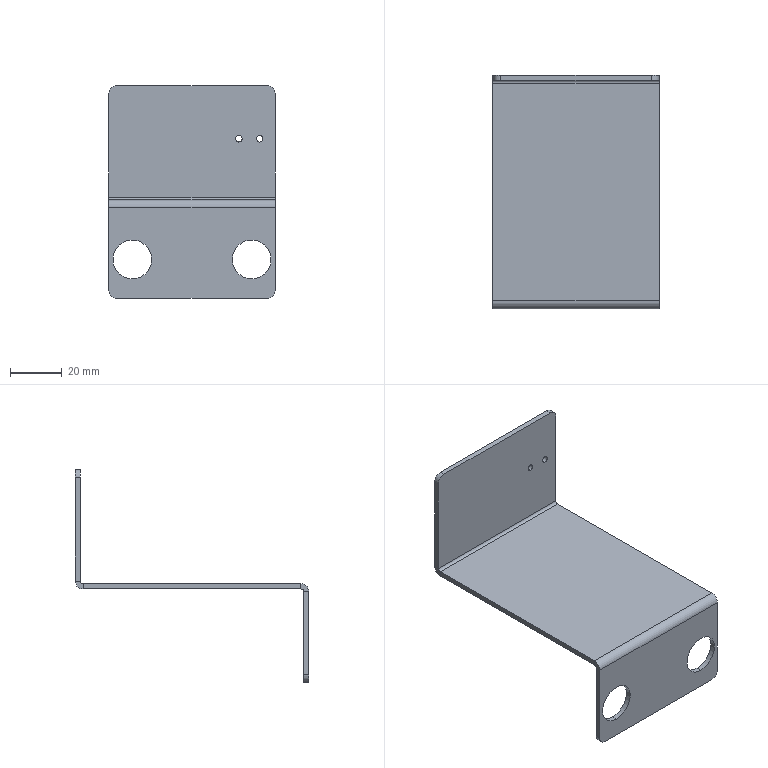Part | STEP file | 001-010-Waste drag chain bracket | 1 solid | 34 faces | box 64 x 90 x 82 mm | volume 20798 mm3 | plane 18 | cylinder 16 | commonest cylinder face diameters 6 x6 2.5 x4 15 x4 2 x2